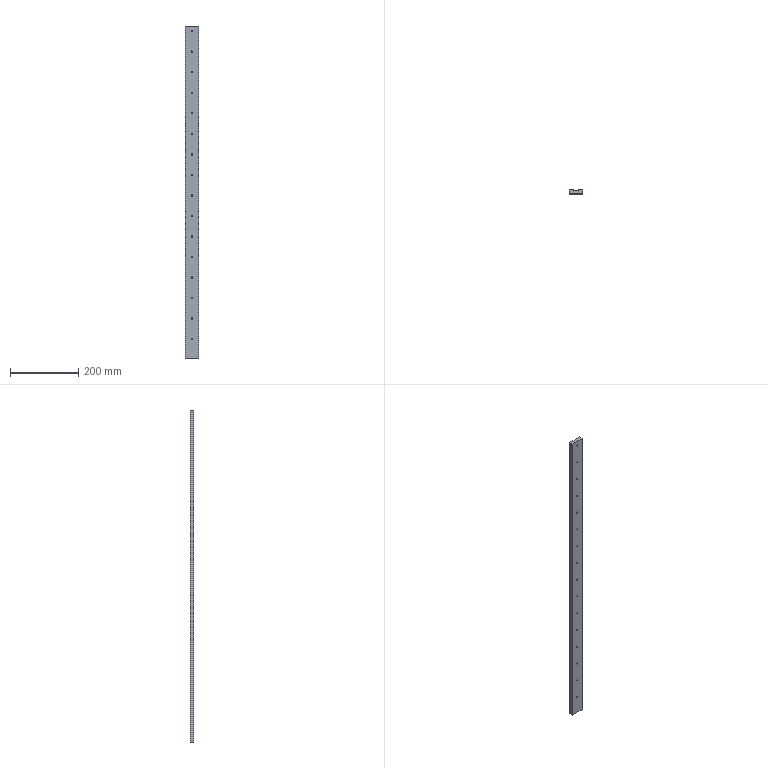Part | STEP file | X77-04205 | 1 solid | 42 faces | box 40 x 11 x 970 mm | volume 388716 mm3 | cylinder 32 | plane 10 | commonest cylinder face diameters 4 x32
STEP:
#1=CARTESIAN_POINT('',(-2.973,12.577,53.));
#2=VERTEX_POINT('',#1);
#3=CARTESIAN_POINT('',(-2.973,12.577,57.));
#4=VERTEX_POINT('',#3);
#5=CARTESIAN_POINT('',(-2.973,12.577,55.));
#6=DIRECTION('',(0.,1.,0.));
#7=DIRECTION('',(0.,0.,1.));
#8=AXIS2_PLACEMENT_3D('',#5,#6,#7);
#9=CIRCLE('',#8,2.);
#10=EDGE_CURVE('',#2,#4,#9,.T.);
#11=ORIENTED_EDGE('',*,*,#10,.F.);
#12=CARTESIAN_POINT('',(-2.973,21.077,53.));
#13=VERTEX_POINT('',#12);
#14=CARTESIAN_POINT('',(-2.973,21.077,53.));
#15=DIRECTION('',(0.,1.,0.));
#16=VECTOR('',#15,1000.);
#17=LINE('',#14,#16);
#18=EDGE_CURVE('',#2,#13,#17,.T.);
#19=ORIENTED_EDGE('',*,*,#18,.T.);
#20=CARTESIAN_POINT('',(-2.973,21.077,57.));
#21=VERTEX_POINT('',#20);
#22=CARTESIAN_POINT('',(-2.973,21.077,55.));
#23=DIRECTION('',(0.,1.,0.));
#24=DIRECTION('',(0.,0.,1.));
#25=AXIS2_PLACEMENT_3D('',#22,#23,#24);
#26=CIRCLE('',#25,2.);
#27=EDGE_CURVE('',#13,#21,#26,.T.);
#28=ORIENTED_EDGE('',*,*,#27,.T.);
#29=CARTESIAN_POINT('',(-2.973,21.077,57.));
#30=DIRECTION('',(0.,1.,0.));
#31=VECTOR('',#30,1000.);
#32=LINE('',#29,#31);
#33=EDGE_CURVE('',#4,#21,#32,.T.);
#34=ORIENTED_EDGE('',*,*,#33,.F.);
#35=EDGE_LOOP('',(#11,#19,#28,#34));
#36=FACE_OUTER_BOUND('',#35,.T.);
#37=CARTESIAN_POINT('',(-2.973,21.077,55.));
#38=DIRECTION('',(0.,1.,0.));
#39=DIRECTION('',(0.,0.,1.));
#40=AXIS2_PLACEMENT_3D('',#37,#38,#39);
#41=CYLINDRICAL_SURFACE('',#40,2.);
#42=ADVANCED_FACE('',(#36),#41,.F.);
#43=CARTESIAN_POINT('',(-2.973,12.577,113.));
#44=VERTEX_POINT('',#43);
#45=CARTESIAN_POINT('',(-2.973,12.577,117.));
#46=VERTEX_POINT('',#45);
#47=CARTESIAN_POINT('',(-2.973,12.577,115.));
#48=DIRECTION('',(0.,1.,0.));
#49=DIRECTION('',(0.,0.,1.));
#50=AXIS2_PLACEMENT_3D('',#47,#48,#49);
#51=CIRCLE('',#50,2.);
#52=EDGE_CURVE('',#44,#46,#51,.T.);
#53=ORIENTED_EDGE('',*,*,#52,.F.);
#54=CARTESIAN_POINT('',(-2.973,21.077,113.));
#55=VERTEX_POINT('',#54);
#56=CARTESIAN_POINT('',(-2.973,21.077,113.));
#57=DIRECTION('',(0.,1.,0.));
#58=VECTOR('',#57,1000.);
#59=LINE('',#56,#58);
#60=EDGE_CURVE('',#44,#55,#59,.T.);
#61=ORIENTED_EDGE('',*,*,#60,.T.);
#62=CARTESIAN_POINT('',(-2.973,21.077,117.));
#63=VERTEX_POINT('',#62);
#64=CARTESIAN_POINT('',(-2.973,21.077,115.));
#65=DIRECTION('',(0.,1.,0.));
#66=DIRECTION('',(0.,0.,1.));
#67=AXIS2_PLACEMENT_3D('',#64,#65,#66);
#68=CIRCLE('',#67,2.);
#69=EDGE_CURVE('',#55,#63,#68,.T.);
#70=ORIENTED_EDGE('',*,*,#69,.T.);
#71=CARTESIAN_POINT('',(-2.973,21.077,117.));
#72=DIRECTION('',(0.,1.,0.));
#73=VECTOR('',#72,1000.);
#74=LINE('',#71,#73);
#75=EDGE_CURVE('',#46,#63,#74,.T.);
#76=ORIENTED_EDGE('',*,*,#75,.F.);
#77=EDGE_LOOP('',(#53,#61,#70,#76));
#78=FACE_OUTER_BOUND('',#77,.T.);
#79=CARTESIAN_POINT('',(-2.973,21.077,115.));
#80=DIRECTION('',(0.,1.,0.));
#81=DIRECTION('',(0.,0.,1.));
#82=AXIS2_PLACEMENT_3D('',#79,#80,#81);
#83=CYLINDRICAL_SURFACE('',#82,2.);
#84=ADVANCED_FACE('',(#78),#83,.F.);
#85=CARTESIAN_POINT('',(-2.973,12.577,173.));
#86=VERTEX_POINT('',#85);
#87=CARTESIAN_POINT('',(-2.973,12.577,177.));
#88=VERTEX_POINT('',#87);
#89=CARTESIAN_POINT('',(-2.973,12.577,175.));
#90=DIRECTION('',(0.,1.,0.));
#91=DIRECTION('',(0.,0.,1.));
#92=AXIS2_PLACEMENT_3D('',#89,#90,#91);
#93=CIRCLE('',#92,2.);
#94=EDGE_CURVE('',#86,#88,#93,.T.);
#95=ORIENTED_EDGE('',*,*,#94,.F.);
#96=CARTESIAN_POINT('',(-2.973,21.077,173.));
#97=VERTEX_POINT('',#96);
#98=CARTESIAN_POINT('',(-2.973,21.077,173.));
#99=DIRECTION('',(0.,1.,0.));
#100=VECTOR('',#99,1000.);
#101=LINE('',#98,#100);
#102=EDGE_CURVE('',#86,#97,#101,.T.);
#103=ORIENTED_EDGE('',*,*,#102,.T.);
#104=CARTESIAN_POINT('',(-2.973,21.077,177.));
#105=VERTEX_POINT('',#104);
#106=CARTESIAN_POINT('',(-2.973,21.077,175.));
#107=DIRECTION('',(0.,1.,0.));
#108=DIRECTION('',(0.,0.,1.));
#109=AXIS2_PLACEMENT_3D('',#106,#107,#108);
#110=CIRCLE('',#109,2.);
#111=EDGE_CURVE('',#97,#105,#110,.T.);
#112=ORIENTED_EDGE('',*,*,#111,.T.);
#113=CARTESIAN_POINT('',(-2.973,21.077,177.));
#114=DIRECTION('',(0.,1.,0.));
#115=VECTOR('',#114,1000.);
#116=LINE('',#113,#115);
#117=EDGE_CURVE('',#88,#105,#116,.T.);
#118=ORIENTED_EDGE('',*,*,#117,.F.);
#119=EDGE_LOOP('',(#95,#103,#112,#118));
#120=FACE_OUTER_BOUND('',#119,.T.);
#121=CARTESIAN_POINT('',(-2.973,21.077,175.));
#122=DIRECTION('',(0.,1.,0.));
#123=DIRECTION('',(0.,0.,1.));
#124=AXIS2_PLACEMENT_3D('',#121,#122,#123);
#125=CYLINDRICAL_SURFACE('',#124,2.);
#126=ADVANCED_FACE('',(#120),#125,.F.);
#127=CARTESIAN_POINT('',(-2.973,12.577,233.));
#128=VERTEX_POINT('',#127);
#129=CARTESIAN_POINT('',(-2.973,12.577,237.));
#130=VERTEX_POINT('',#129);
#131=CARTESIAN_POINT('',(-2.973,12.577,235.));
#132=DIRECTION('',(0.,1.,0.));
#133=DIRECTION('',(0.,0.,1.));
#134=AXIS2_PLACEMENT_3D('',#131,#132,#133);
#135=CIRCLE('',#134,2.);
#136=EDGE_CURVE('',#128,#130,#135,.T.);
#137=ORIENTED_EDGE('',*,*,#136,.F.);
#138=CARTESIAN_POINT('',(-2.973,21.077,233.));
#139=VERTEX_POINT('',#138);
#140=CARTESIAN_POINT('',(-2.973,21.077,233.));
#141=DIRECTION('',(0.,1.,0.));
#142=VECTOR('',#141,1000.);
#143=LINE('',#140,#142);
#144=EDGE_CURVE('',#128,#139,#143,.T.);
#145=ORIENTED_EDGE('',*,*,#144,.T.);
#146=CARTESIAN_POINT('',(-2.973,21.077,237.));
#147=VERTEX_POINT('',#146);
#148=CARTESIAN_POINT('',(-2.973,21.077,235.));
#149=DIRECTION('',(0.,1.,0.));
#150=DIRECTION('',(0.,0.,1.));
#151=AXIS2_PLACEMENT_3D('',#148,#149,#150);
#152=CIRCLE('',#151,2.);
#153=EDGE_CURVE('',#139,#147,#152,.T.);
#154=ORIENTED_EDGE('',*,*,#153,.T.);
#155=CARTESIAN_POINT('',(-2.973,21.077,237.));
#156=DIRECTION('',(0.,1.,0.));
#157=VECTOR('',#156,1000.);
#158=LINE('',#155,#157);
#159=EDGE_CURVE('',#130,#147,#158,.T.);
#160=ORIENTED_EDGE('',*,*,#159,.F.);
#161=EDGE_LOOP('',(#137,#145,#154,#160));
#162=FACE_OUTER_BOUND('',#161,.T.);
#163=CARTESIAN_POINT('',(-2.973,21.077,235.));
#164=DIRECTION('',(0.,1.,0.));
#165=DIRECTION('',(0.,0.,1.));
#166=AXIS2_PLACEMENT_3D('',#163,#164,#165);
#167=CYLINDRICAL_SURFACE('',#166,2.);
#168=ADVANCED_FACE('',(#162),#167,.F.);
#169=CARTESIAN_POINT('',(-2.973,12.577,293.));
#170=VERTEX_POINT('',#169);
#171=CARTESIAN_POINT('',(-2.973,12.577,297.));
#172=VERTEX_POINT('',#171);
#173=CARTESIAN_POINT('',(-2.973,12.577,295.));
#174=DIRECTION('',(0.,1.,0.));
#175=DIRECTION('',(0.,0.,1.));
#176=AXIS2_PLACEMENT_3D('',#173,#174,#175);
#177=CIRCLE('',#176,2.);
#178=EDGE_CURVE('',#170,#172,#177,.T.);
#179=ORIENTED_EDGE('',*,*,#178,.F.);
#180=CARTESIAN_POINT('',(-2.973,21.077,293.));
#181=VERTEX_POINT('',#180);
#182=CARTESIAN_POINT('',(-2.973,21.077,293.));
#183=DIRECTION('',(0.,1.,0.));
#184=VECTOR('',#183,1000.);
#185=LINE('',#182,#184);
#186=EDGE_CURVE('',#170,#181,#185,.T.);
#187=ORIENTED_EDGE('',*,*,#186,.T.);
#188=CARTESIAN_POINT('',(-2.973,21.077,297.));
#189=VERTEX_POINT('',#188);
#190=CARTESIAN_POINT('',(-2.973,21.077,295.));
#191=DIRECTION('',(0.,1.,0.));
#192=DIRECTION('',(0.,0.,1.));
#193=AXIS2_PLACEMENT_3D('',#190,#191,#192);
#194=CIRCLE('',#193,2.);
#195=EDGE_CURVE('',#181,#189,#194,.T.);
#196=ORIENTED_EDGE('',*,*,#195,.T.);
#197=CARTESIAN_POINT('',(-2.973,21.077,297.));
#198=DIRECTION('',(0.,1.,0.));
#199=VECTOR('',#198,1000.);
#200=LINE('',#197,#199);
#201=EDGE_CURVE('',#172,#189,#200,.T.);
#202=ORIENTED_EDGE('',*,*,#201,.F.);
#203=EDGE_LOOP('',(#179,#187,#196,#202));
#204=FACE_OUTER_BOUND('',#203,.T.);
#205=CARTESIAN_POINT('',(-2.973,21.077,295.));
#206=DIRECTION('',(0.,1.,0.));
#207=DIRECTION('',(0.,0.,1.));
#208=AXIS2_PLACEMENT_3D('',#205,#206,#207);
#209=CYLINDRICAL_SURFACE('',#208,2.);
#210=ADVANCED_FACE('',(#204),#209,.F.);
#211=CARTESIAN_POINT('',(-2.973,12.577,353.));
#212=VERTEX_POINT('',#211);
#213=CARTESIAN_POINT('',(-2.973,12.577,357.));
#214=VERTEX_POINT('',#213);
#215=CARTESIAN_POINT('',(-2.973,12.577,355.));
#216=DIRECTION('',(0.,1.,0.));
#217=DIRECTION('',(0.,0.,1.));
#218=AXIS2_PLACEMENT_3D('',#215,#216,#217);
#219=CIRCLE('',#218,2.);
#220=EDGE_CURVE('',#212,#214,#219,.T.);
#221=ORIENTED_EDGE('',*,*,#220,.F.);
#222=CARTESIAN_POINT('',(-2.973,21.077,353.));
#223=VERTEX_POINT('',#222);
#224=CARTESIAN_POINT('',(-2.973,21.077,353.));
#225=DIRECTION('',(0.,1.,0.));
#226=VECTOR('',#225,1000.);
#227=LINE('',#224,#226);
#228=EDGE_CURVE('',#212,#223,#227,.T.);
#229=ORIENTED_EDGE('',*,*,#228,.T.);
#230=CARTESIAN_POINT('',(-2.973,21.077,357.));
#231=VERTEX_POINT('',#230);
#232=CARTESIAN_POINT('',(-2.973,21.077,355.));
#233=DIRECTION('',(0.,1.,0.));
#234=DIRECTION('',(0.,0.,1.));
#235=AXIS2_PLACEMENT_3D('',#232,#233,#234);
#236=CIRCLE('',#235,2.);
#237=EDGE_CURVE('',#223,#231,#236,.T.);
#238=ORIENTED_EDGE('',*,*,#237,.T.);
#239=CARTESIAN_POINT('',(-2.973,21.077,357.));
#240=DIRECTION('',(0.,1.,0.));
#241=VECTOR('',#240,1000.);
#242=LINE('',#239,#241);
#243=EDGE_CURVE('',#214,#231,#242,.T.);
#244=ORIENTED_EDGE('',*,*,#243,.F.);
#245=EDGE_LOOP('',(#221,#229,#238,#244));
#246=FACE_OUTER_BOUND('',#245,.T.);
#247=CARTESIAN_POINT('',(-2.973,21.077,355.));
#248=DIRECTION('',(0.,1.,0.));
#249=DIRECTION('',(0.,0.,1.));
#250=AXIS2_PLACEMENT_3D('',#247,#248,#249);
#251=CYLINDRICAL_SURFACE('',#250,2.);
#252=ADVANCED_FACE('',(#246),#251,.F.);
#253=CARTESIAN_POINT('',(-2.973,12.577,413.));
#254=VERTEX_POINT('',#253);
#255=CARTESIAN_POINT('',(-2.973,12.577,417.));
#256=VERTEX_POINT('',#255);
#257=CARTESIAN_POINT('',(-2.973,12.577,415.));
#258=DIRECTION('',(0.,1.,0.));
#259=DIRECTION('',(0.,0.,1.));
#260=AXIS2_PLACEMENT_3D('',#257,#258,#259);
#261=CIRCLE('',#260,2.);
#262=EDGE_CURVE('',#254,#256,#261,.T.);
#263=ORIENTED_EDGE('',*,*,#262,.F.);
#264=CARTESIAN_POINT('',(-2.973,21.077,413.));
#265=VERTEX_POINT('',#264);
#266=CARTESIAN_POINT('',(-2.973,21.077,413.));
#267=DIRECTION('',(0.,1.,0.));
#268=VECTOR('',#267,1000.);
#269=LINE('',#266,#268);
#270=EDGE_CURVE('',#254,#265,#269,.T.);
#271=ORIENTED_EDGE('',*,*,#270,.T.);
#272=CARTESIAN_POINT('',(-2.973,21.077,417.));
#273=VERTEX_POINT('',#272);
#274=CARTESIAN_POINT('',(-2.973,21.077,415.));
#275=DIRECTION('',(0.,1.,0.));
#276=DIRECTION('',(0.,0.,1.));
#277=AXIS2_PLACEMENT_3D('',#274,#275,#276);
#278=CIRCLE('',#277,2.);
#279=EDGE_CURVE('',#265,#273,#278,.T.);
#280=ORIENTED_EDGE('',*,*,#279,.T.);
#281=CARTESIAN_POINT('',(-2.973,21.077,417.));
#282=DIRECTION('',(0.,1.,0.));
#283=VECTOR('',#282,1000.);
#284=LINE('',#281,#283);
#285=EDGE_CURVE('',#256,#273,#284,.T.);
#286=ORIENTED_EDGE('',*,*,#285,.F.);
#287=EDGE_LOOP('',(#263,#271,#280,#286));
#288=FACE_OUTER_BOUND('',#287,.T.);
#289=CARTESIAN_POINT('',(-2.973,21.077,415.));
#290=DIRECTION('',(0.,1.,0.));
#291=DIRECTION('',(0.,0.,1.));
#292=AXIS2_PLACEMENT_3D('',#289,#290,#291);
#293=CYLINDRICAL_SURFACE('',#292,2.);
#294=ADVANCED_FACE('',(#288),#293,.F.);
#295=CARTESIAN_POINT('',(-2.973,12.577,473.));
#296=VERTEX_POINT('',#295);
#297=CARTESIAN_POINT('',(-2.973,12.577,477.));
#298=VERTEX_POINT('',#297);
#299=CARTESIAN_POINT('',(-2.973,12.577,475.));
#300=DIRECTION('',(0.,1.,0.));
#301=DIRECTION('',(0.,0.,1.));
#302=AXIS2_PLACEMENT_3D('',#299,#300,#301);
#303=CIRCLE('',#302,2.);
#304=EDGE_CURVE('',#296,#298,#303,.T.);
#305=ORIENTED_EDGE('',*,*,#304,.F.);
#306=CARTESIAN_POINT('',(-2.973,21.077,473.));
#307=VERTEX_POINT('',#306);
#308=CARTESIAN_POINT('',(-2.973,21.077,473.));
#309=DIRECTION('',(0.,1.,0.));
#310=VECTOR('',#309,1000.);
#311=LINE('',#308,#310);
#312=EDGE_CURVE('',#296,#307,#311,.T.);
#313=ORIENTED_EDGE('',*,*,#312,.T.);
#314=CARTESIAN_POINT('',(-2.973,21.077,477.));
#315=VERTEX_POINT('',#314);
#316=CARTESIAN_POINT('',(-2.973,21.077,475.));
#317=DIRECTION('',(0.,1.,0.));
#318=DIRECTION('',(0.,0.,1.));
#319=AXIS2_PLACEMENT_3D('',#316,#317,#318);
#320=CIRCLE('',#319,2.);
#321=EDGE_CURVE('',#307,#315,#320,.T.);
#322=ORIENTED_EDGE('',*,*,#321,.T.);
#323=CARTESIAN_POINT('',(-2.973,21.077,477.));
#324=DIRECTION('',(0.,1.,0.));
#325=VECTOR('',#324,1000.);
#326=LINE('',#323,#325);
#327=EDGE_CURVE('',#298,#315,#326,.T.);
#328=ORIENTED_EDGE('',*,*,#327,.F.);
#329=EDGE_LOOP('',(#305,#313,#322,#328));
#330=FACE_OUTER_BOUND('',#329,.T.);
#331=CARTESIAN_POINT('',(-2.973,21.077,475.));
#332=DIRECTION('',(0.,1.,0.));
#333=DIRECTION('',(0.,0.,1.));
#334=AXIS2_PLACEMENT_3D('',#331,#332,#333);
#335=CYLINDRICAL_SURFACE('',#334,2.);
#336=ADVANCED_FACE('',(#330),#335,.F.);
#337=CARTESIAN_POINT('',(-2.973,12.577,533.));
#338=VERTEX_POINT('',#337);
#339=CARTESIAN_POINT('',(-2.973,12.577,537.));
#340=VERTEX_POINT('',#339);
#341=CARTESIAN_POINT('',(-2.973,12.577,535.));
#342=DIRECTION('',(0.,1.,0.));
#343=DIRECTION('',(0.,0.,1.));
#344=AXIS2_PLACEMENT_3D('',#341,#342,#343);
#345=CIRCLE('',#344,2.);
#346=EDGE_CURVE('',#338,#340,#345,.T.);
#347=ORIENTED_EDGE('',*,*,#346,.F.);
#348=CARTESIAN_POINT('',(-2.973,21.077,533.));
#349=VERTEX_POINT('',#348);
#350=CARTESIAN_POINT('',(-2.973,21.077,533.));
#351=DIRECTION('',(0.,1.,0.));
#352=VECTOR('',#351,1000.);
#353=LINE('',#350,#352);
#354=EDGE_CURVE('',#338,#349,#353,.T.);
#355=ORIENTED_EDGE('',*,*,#354,.T.);
#356=CARTESIAN_POINT('',(-2.973,21.077,537.));
#357=VERTEX_POINT('',#356);
#358=CARTESIAN_POINT('',(-2.973,21.077,535.));
#359=DIRECTION('',(0.,1.,0.));
#360=DIRECTION('',(0.,0.,1.));
#361=AXIS2_PLACEMENT_3D('',#358,#359,#360);
#362=CIRCLE('',#361,2.);
#363=EDGE_CURVE('',#349,#357,#362,.T.);
#364=ORIENTED_EDGE('',*,*,#363,.T.);
#365=CARTESIAN_POINT('',(-2.973,21.077,537.));
#366=DIRECTION('',(0.,1.,0.));
#367=VECTOR('',#366,1000.);
#368=LINE('',#365,#367);
#369=EDGE_CURVE('',#340,#357,#368,.T.);
#370=ORIENTED_EDGE('',*,*,#369,.F.);
#371=EDGE_LOOP('',(#347,#355,#364,#370));
#372=FACE_OUTER_BOUND('',#371,.T.);
#373=CARTESIAN_POINT('',(-2.973,21.077,535.));
#374=DIRECTION('',(0.,1.,0.));
#375=DIRECTION('',(0.,0.,1.));
#376=AXIS2_PLACEMENT_3D('',#373,#374,#375);
#377=CYLINDRICAL_SURFACE('',#376,2.);
#378=ADVANCED_FACE('',(#372),#377,.F.);
#379=CARTESIAN_POINT('',(-2.973,12.577,593.));
#380=VERTEX_POINT('',#379);
#381=CARTESIAN_POINT('',(-2.973,12.577,597.));
#382=VERTEX_POINT('',#381);
#383=CARTESIAN_POINT('',(-2.973,12.577,595.));
#384=DIRECTION('',(0.,1.,0.));
#385=DIRECTION('',(0.,0.,1.));
#386=AXIS2_PLACEMENT_3D('',#383,#384,#385);
#387=CIRCLE('',#386,2.);
#388=EDGE_CURVE('',#380,#382,#387,.T.);
#389=ORIENTED_EDGE('',*,*,#388,.F.);
#390=CARTESIAN_POINT('',(-2.973,21.077,593.));
#391=VERTEX_POINT('',#390);
#392=CARTESIAN_POINT('',(-2.973,21.077,593.));
#393=DIRECTION('',(0.,1.,0.));
#394=VECTOR('',#393,1000.);
#395=LINE('',#392,#394);
#396=EDGE_CURVE('',#380,#391,#395,.T.);
#397=ORIENTED_EDGE('',*,*,#396,.T.);
#398=CARTESIAN_POINT('',(-2.973,21.077,597.));
#399=VERTEX_POINT('',#398);
#400=CARTESIAN_POINT('',(-2.973,21.077,595.));
#401=DIRECTION('',(0.,1.,0.));
#402=DIRECTION('',(0.,0.,1.));
#403=AXIS2_PLACEMENT_3D('',#400,#401,#402);
#404=CIRCLE('',#403,2.);
#405=EDGE_CURVE('',#391,#399,#404,.T.);
#406=ORIENTED_EDGE('',*,*,#405,.T.);
#407=CARTESIAN_POINT('',(-2.973,21.077,597.));
#408=DIRECTION('',(0.,1.,0.));
#409=VECTOR('',#408,1000.);
#410=LINE('',#407,#409);
#411=EDGE_CURVE('',#382,#399,#410,.T.);
#412=ORIENTED_EDGE('',*,*,#411,.F.);
#413=EDGE_LOOP('',(#389,#397,#406,#412));
#414=FACE_OUTER_BOUND('',#413,.T.);
#415=CARTESIAN_POINT('',(-2.973,21.077,595.));
#416=DIRECTION('',(0.,1.,0.));
#417=DIRECTION('',(0.,0.,1.));
#418=AXIS2_PLACEMENT_3D('',#415,#416,#417);
#419=CYLINDRICAL_SURFACE('',#418,2.);
#420=ADVANCED_FACE('',(#414),#419,.F.);
#421=CARTESIAN_POINT('',(-2.973,12.577,653.));
#422=VERTEX_POINT('',#421);
#423=CARTESIAN_POINT('',(-2.973,12.577,657.));
#424=VERTEX_POINT('',#423);
#425=CARTESIAN_POINT('',(-2.973,12.577,655.));
#426=DIRECTION('',(0.,1.,0.));
#427=DIRECTION('',(0.,0.,1.));
#428=AXIS2_PLACEMENT_3D('',#425,#426,#427);
#429=CIRCLE('',#428,2.);
#430=EDGE_CURVE('',#422,#424,#429,.T.);
#431=ORIENTED_EDGE('',*,*,#430,.F.);
#432=CARTESIAN_POINT('',(-2.973,21.077,653.));
#433=VERTEX_POINT('',#432);
#434=CARTESIAN_POINT('',(-2.973,21.077,653.));
#435=DIRECTION('',(0.,1.,0.));
#436=VECTOR('',#435,1000.);
#437=LINE('',#434,#436);
#438=EDGE_CURVE('',#422,#433,#437,.T.);
#439=ORIENTED_EDGE('',*,*,#438,.T.);
#440=CARTESIAN_POINT('',(-2.973,21.077,657.));
#441=VERTEX_POINT('',#440);
#442=CARTESIAN_POINT('',(-2.973,21.077,655.));
#443=DIRECTION('',(0.,1.,0.));
#444=DIRECTION('',(0.,0.,1.));
#445=AXIS2_PLACEMENT_3D('',#442,#443,#444);
#446=CIRCLE('',#445,2.);
#447=EDGE_CURVE('',#433,#441,#446,.T.);
#448=ORIENTED_EDGE('',*,*,#447,.T.);
#449=CARTESIAN_POINT('',(-2.973,21.077,657.));
#450=DIRECTION('',(0.,1.,0.));
#451=VECTOR('',#450,1000.);
#452=LINE('',#449,#451);
#453=EDGE_CURVE('',#424,#441,#452,.T.);
#454=ORIENTED_EDGE('',*,*,#453,.F.);
#455=EDGE_LOOP('',(#431,#439,#448,#454));
#456=FACE_OUTER_BOUND('',#455,.T.);
#457=CARTESIAN_POINT('',(-2.973,21.077,655.));
#458=DIRECTION('',(0.,1.,0.));
#459=DIRECTION('',(0.,0.,1.));
#460=AXIS2_PLACEMENT_3D('',#457,#458,#459);
#461=CYLINDRICAL_SURFACE('',#460,2.);
#462=ADVANCED_FACE('',(#456),#461,.F.);
#463=CARTESIAN_POINT('',(-2.973,12.577,713.));
#464=VERTEX_POINT('',#463);
#465=CARTESIAN_POINT('',(-2.973,12.577,717.));
#466=VERTEX_POINT('',#465);
#467=CARTESIAN_POINT('',(-2.973,12.577,715.));
#468=DIRECTION('',(0.,1.,0.));
#469=DIRECTION('',(0.,0.,1.));
#470=AXIS2_PLACEMENT_3D('',#467,#468,#469);
#471=CIRCLE('',#470,2.);
#472=EDGE_CURVE('',#464,#466,#471,.T.);
#473=ORIENTED_EDGE('',*,*,#472,.F.);
#474=CARTESIAN_POINT('',(-2.973,21.077,713.));
#475=VERTEX_POINT('',#474);
#476=CARTESIAN_POINT('',(-2.973,21.077,713.));
#477=DIRECTION('',(0.,1.,0.));
#478=VECTOR('',#477,1000.);
#479=LINE('',#476,#478);
#480=EDGE_CURVE('',#464,#475,#479,.T.);
#481=ORIENTED_EDGE('',*,*,#480,.T.);
#482=CARTESIAN_POINT('',(-2.973,21.077,717.));
#483=VERTEX_POINT('',#482);
#484=CARTESIAN_POINT('',(-2.973,21.077,715.));
#485=DIRECTION('',(0.,1.,0.));
#486=DIRECTION('',(0.,0.,1.));
#487=AXIS2_PLACEMENT_3D('',#484,#485,#486);
#488=CIRCLE('',#487,2.);
#489=EDGE_CURVE('',#475,#483,#488,.T.);
#490=ORIENTED_EDGE('',*,*,#489,.T.);
#491=CARTESIAN_POINT('',(-2.973,21.077,717.));
#492=DIRECTION('',(0.,1.,0.));
#493=VECTOR('',#492,1000.);
#494=LINE('',#491,#493);
#495=EDGE_CURVE('',#466,#483,#494,.T.);
#496=ORIENTED_EDGE('',*,*,#495,.F.);
#497=EDGE_LOOP('',(#473,#481,#490,#496));
#498=FACE_OUTER_BOUND('',#497,.T.);
#499=CARTESIAN_POINT('',(-2.973,21.077,715.));
#500=DIRECTION('',(0.,1.,0.));
#501=DIRECTION('',(0.,0.,1.));
#502=AXIS2_PLACEMENT_3D('',#499,#500,#501);
#503=CYLINDRICAL_SURFACE('',#502,2.);
#504=ADVANCED_FACE('',(#498),#503,.F.);
#505=CARTESIAN_POINT('',(-2.973,12.577,773.));
#506=VERTEX_POINT('',#505);
#507=CARTESIAN_POINT('',(-2.973,12.577,777.));
#508=VERTEX_POINT('',#507);
#509=CARTESIAN_POINT('',(-2.973,12.577,775.));
#510=DIRECTION('',(0.,1.,0.));
#511=DIRECTION('',(0.,0.,1.));
#512=AXIS2_PLACEMENT_3D('',#509,#510,#511);
#513=CIRCLE('',#512,2.);
#514=EDGE_CURVE('',#506,#508,#513,.T.);
#515=ORIENTED_EDGE('',*,*,#514,.F.);
#516=CARTESIAN_POINT('',(-2.973,21.077,773.));
#517=VERTEX_POINT('',#516);
#518=CARTESIAN_POINT('',(-2.973,21.077,773.));
#519=DIRECTION('',(0.,1.,0.));
#520=VECTOR('',#519,1000.);
#521=LINE('',#518,#520);
#522=EDGE_CURVE('',#506,#517,#521,.T.);
#523=ORIENTED_EDGE('',*,*,#522,.T.);
#524=CARTESIAN_POINT('',(-2.973,21.077,777.));
#525=VERTEX_POINT('',#524);
#526=CARTESIAN_POINT('',(-2.973,21.077,775.));
#527=DIRECTION('',(0.,1.,0.));
#528=DIRECTION('',(0.,0.,1.));
#529=AXIS2_PLACEMENT_3D('',#526,#527,#528);
#530=CIRCLE('',#529,2.);
#531=EDGE_CURVE('',#517,#525,#530,.T.);
#532=ORIENTED_EDGE('',*,*,#531,.T.);
#533=CARTESIAN_POINT('',(-2.973,21.077,777.));
#534=DIRECTION('',(0.,1.,0.));
#535=VECTOR('',#534,1000.);
#536=LINE('',#533,#535);
#537=EDGE_CURVE('',#508,#525,#536,.T.);
#538=ORIENTED_EDGE('',*,*,#537,.F.);
#539=EDGE_LOOP('',(#515,#523,#532,#538));
#540=FACE_OUTER_BOUND('',#539,.T.);
#541=CARTESIAN_POINT('',(-2.973,21.077,775.));
#542=DIRECTION('',(0.,1.,0.));
#543=DIRECTION('',(0.,0.,1.));
#544=AXIS2_PLACEMENT_3D('',#541,#542,#543);
#545=CYLINDRICAL_SURFACE('',#544,2.);
#546=ADVANCED_FACE('',(#540),#545,.F.);
#547=CARTESIAN_POINT('',(-2.973,12.577,833.));
#548=VERTEX_POINT('',#547);
#549=CARTESIAN_POINT('',(-2.973,12.577,837.));
#550=VERTEX_POINT('',#549);
#551=CARTESIAN_POINT('',(-2.973,12.577,835.));
#552=DIRECTION('',(0.,1.,0.));
#553=DIRECTION('',(0.,0.,1.));
#554=AXIS2_PLACEMENT_3D('',#551,#552,#553);
#555=CIRCLE('',#554,2.);
#556=EDGE_CURVE('',#548,#550,#555,.T.);
#557=ORIENTED_EDGE('',*,*,#556,.F.);
#558=CARTESIAN_POINT('',(-2.973,21.077,833.));
#559=VERTEX_POINT('',#558);
#560=CARTESIAN_POINT('',(-2.973,21.077,833.));
#561=DIRECTION('',(0.,1.,0.));
#562=VECTOR('',#561,1000.);
#563=LINE('',#560,#562);
#564=EDGE_CURVE('',#548,#559,#563,.T.);
#565=ORIENTED_EDGE('',*,*,#564,.T.);
#566=CARTESIAN_POINT('',(-2.973,21.077,837.));
#567=VERTEX_POINT('',#566);
#568=CARTESIAN_POINT('',(-2.973,21.077,835.));
#569=DIRECTION('',(0.,1.,0.));
#570=DIRECTION('',(0.,0.,1.));
#571=AXIS2_PLACEMENT_3D('',#568,#569,#570);
#572=CIRCLE('',#571,2.);
#573=EDGE_CURVE('',#559,#567,#572,.T.);
#574=ORIENTED_EDGE('',*,*,#573,.T.);
#575=CARTESIAN_POINT('',(-2.973,21.077,837.));
#576=DIRECTION('',(0.,1.,0.));
#577=VECTOR('',#576,1000.);
#578=LINE('',#575,#577);
#579=EDGE_CURVE('',#550,#567,#578,.T.);
#580=ORIENTED_EDGE('',*,*,#579,.F.);
#581=EDGE_LOOP('',(#557,#565,#574,#580));
#582=FACE_OUTER_BOUND('',#581,.T.);
#583=CARTESIAN_POINT('',(-2.973,21.077,835.));
#584=DIRECTION('',(0.,1.,0.));
#585=DIRECTION('',(0.,0.,1.));
#586=AXIS2_PLACEMENT_3D('',#583,#584,#585);
#587=CYLINDRICAL_SURFACE('',#586,2.);
#588=ADVANCED_FACE('',(#582),#587,.F.);
#589=CARTESIAN_POINT('',(-2.973,12.577,893.));
#590=VERTEX_POINT('',#589);
#591=CARTESIAN_POINT('',(-2.973,12.577,897.));
#592=VERTEX_POINT('',#591);
#593=CARTESIAN_POINT('',(-2.973,12.577,895.));
#594=DIRECTION('',(0.,1.,0.));
#595=DIRECTION('',(0.,0.,1.));
#596=AXIS2_PLACEMENT_3D('',#593,#594,#595);
#597=CIRCLE('',#596,2.);
#598=EDGE_CURVE('',#590,#592,#597,.T.);
#599=ORIENTED_EDGE('',*,*,#598,.F.);
#600=CARTESIAN_POINT('',(-2.973,21.077,893.));
#601=VERTEX_POINT('',#600);
#602=CARTESIAN_POINT('',(-2.973,21.077,893.));
#603=DIRECTION('',(0.,1.,0.));
#604=VECTOR('',#603,1000.);
#605=LINE('',#602,#604);
#606=EDGE_CURVE('',#590,#601,#605,.T.);
#607=ORIENTED_EDGE('',*,*,#606,.T.);
#608=CARTESIAN_POINT('',(-2.973,21.077,897.));
#609=VERTEX_POINT('',#608);
#610=CARTESIAN_POINT('',(-2.973,21.077,895.));
#611=DIRECTION('',(0.,1.,0.));
#612=DIRECTION('',(0.,0.,1.));
#613=AXIS2_PLACEMENT_3D('',#610,#611,#612);
#614=CIRCLE('',#613,2.);
#615=EDGE_CURVE('',#601,#609,#614,.T.);
#616=ORIENTED_EDGE('',*,*,#615,.T.);
#617=CARTESIAN_POINT('',(-2.973,21.077,897.));
#618=DIRECTION('',(0.,1.,0.));
#619=VECTOR('',#618,1000.);
#620=LINE('',#617,#619);
#621=EDGE_CURVE('',#592,#609,#620,.T.);
#622=ORIENTED_EDGE('',*,*,#621,.F.);
#623=EDGE_LOOP('',(#599,#607,#616,#622));
#624=FACE_OUTER_BOUND('',#623,.T.);
#625=CARTESIAN_POINT('',(-2.973,21.077,895.));
#626=DIRECTION('',(0.,1.,0.));
#627=DIRECTION('',(0.,0.,1.));
#628=AXIS2_PLACEMENT_3D('',#625,#626,#627);
#629=CYLINDRICAL_SURFACE('',#628,2.);
#630=ADVANCED_FACE('',(#624),#629,.F.);
#631=CARTESIAN_POINT('',(-2.973,12.577,953.));
#632=VERTEX_POINT('',#631);
#633=CARTESIAN_POINT('',(-2.973,12.577,957.));
#634=VERTEX_POINT('',#633);
#635=CARTESIAN_POINT('',(-2.973,12.577,955.));
#636=DIRECTION('',(0.,1.,0.));
#637=DIRECTION('',(0.,0.,1.));
#638=AXIS2_PLACEMENT_3D('',#635,#636,#637);
#639=CIRCLE('',#638,2.);
#640=EDGE_CURVE('',#632,#634,#639,.T.);
#641=ORIENTED_EDGE('',*,*,#640,.F.);
#642=CARTESIAN_POINT('',(-2.973,21.077,953.));
#643=VERTEX_POINT('',#642);
#644=CARTESIAN_POINT('',(-2.973,21.077,953.));
#645=DIRECTION('',(0.,1.,0.));
#646=VECTOR('',#645,1000.);
#647=LINE('',#644,#646);
#648=EDGE_CURVE('',#632,#643,#647,.T.);
#649=ORIENTED_EDGE('',*,*,#648,.T.);
#650=CARTESIAN_POINT('',(-2.973,21.077,957.));
#651=VERTEX_POINT('',#650);
#652=CARTESIAN_POINT('',(-2.973,21.077,955.));
#653=DIRECTION('',(0.,1.,0.));
#654=DIRECTION('',(0.,0.,1.));
#655=AXIS2_PLACEMENT_3D('',#652,#653,#654);
#656=CIRCLE('',#655,2.);
#657=EDGE_CURVE('',#643,#651,#656,.T.);
#658=ORIENTED_EDGE('',*,*,#657,.T.);
#659=CARTESIAN_POINT('',(-2.973,21.077,957.));
#660=DIRECTION('',(0.,1.,0.));
#661=VECTOR('',#660,1000.);
#662=LINE('',#659,#661);
#663=EDGE_CURVE('',#634,#651,#662,.T.);
#664=ORIENTED_EDGE('',*,*,#663,.F.);
#665=EDGE_LOOP('',(#641,#649,#658,#664));
#666=FACE_OUTER_BOUND('',#665,.T.);
#667=CARTESIAN_POINT('',(-2.973,21.077,955.));
#668=DIRECTION('',(0.,1.,0.));
#669=DIRECTION('',(0.,0.,1.));
#670=AXIS2_PLACEMENT_3D('',#667,#668,#669);
#671=CYLINDRICAL_SURFACE('',#670,2.);
#672=ADVANCED_FACE('',(#666),#671,.F.);
#673=CARTESIAN_POINT('',(17.027,23.577,0.));
#674=VERTEX_POINT('',#673);
#675=CARTESIAN_POINT('',(4.527,23.577,0.));
#676=VERTEX_POINT('',#675);
#677=CARTESIAN_POINT('',(-22.973,23.577,0.));
#678=DIRECTION('',(-1.,0.,0.));
#679=VECTOR('',#678,1000.);
#680=LINE('',#677,#679);
#681=EDGE_CURVE('',#674,#676,#680,.T.);
#682=ORIENTED_EDGE('',*,*,#681,.T.);
#683=CARTESIAN_POINT('',(4.527,23.577,970.));
#684=VERTEX_POINT('',#683);
#685=CARTESIAN_POINT('',(4.527,23.577,0.));
#686=DIRECTION('',(0.,0.,1.));
#687=VECTOR('',#686,1000.);
#688=LINE('',#685,#687);
#689=EDGE_CURVE('',#676,#684,#688,.T.);
#690=ORIENTED_EDGE('',*,*,#689,.T.);
#691=CARTESIAN_POINT('',(17.027,23.577,970.));
#692=VERTEX_POINT('',#691);
#693=CARTESIAN_POINT('',(-22.973,23.577,970.));
#694=DIRECTION('',(-1.,0.,0.));
#695=VECTOR('',#694,1000.);
#696=LINE('',#693,#695);
#697=EDGE_CURVE('',#692,#684,#696,.T.);
#698=ORIENTED_EDGE('',*,*,#697,.F.);
#699=CARTESIAN_POINT('',(17.027,23.577,970.));
#700=DIRECTION('',(0.,0.,-1.));
#701=VECTOR('',#700,1000.);
#702=LINE('',#699,#701);
#703=EDGE_CURVE('',#692,#674,#702,.T.);
#704=ORIENTED_EDGE('',*,*,#703,.T.);
#705=EDGE_LOOP('',(#682,#690,#698,#704));
#706=FACE_OUTER_BOUND('',#705,.T.);
#707=CARTESIAN_POINT('',(-22.973,23.577,970.));
#708=DIRECTION('',(0.,-1.,0.));
#709=DIRECTION('',(0.,0.,-1.));
#710=AXIS2_PLACEMENT_3D('',#707,#708,#709);
#711=PLANE('',#710);
#712=ADVANCED_FACE('',(#706),#711,.F.);
#713=CARTESIAN_POINT('',(-22.973,23.577,0.));
#714=VERTEX_POINT('',#713);
#715=CARTESIAN_POINT('',(-22.973,12.577,0.));
#716=VERTEX_POINT('',#715);
#717=CARTESIAN_POINT('',(-22.973,12.577,0.));
#718=DIRECTION('',(0.,-1.,0.));
#719=VECTOR('',#718,1000.);
#720=LINE('',#717,#719);
#721=EDGE_CURVE('',#714,#716,#720,.T.);
#722=ORIENTED_EDGE('',*,*,#721,.T.);
#723=CARTESIAN_POINT('',(-22.973,12.577,970.));
#724=VERTEX_POINT('',#723);
#725=CARTESIAN_POINT('',(-22.973,12.577,970.));
#726=DIRECTION('',(0.,0.,-1.));
#727=VECTOR('',#726,1000.);
#728=LINE('',#725,#727);
#729=EDGE_CURVE('',#724,#716,#728,.T.);
#730=ORIENTED_EDGE('',*,*,#729,.F.);
#731=CARTESIAN_POINT('',(-22.973,23.577,970.));
#732=VERTEX_POINT('',#731);
#733=CARTESIAN_POINT('',(-22.973,12.577,970.));
#734=DIRECTION('',(0.,-1.,0.));
#735=VECTOR('',#734,1000.);
#736=LINE('',#733,#735);
#737=EDGE_CURVE('',#732,#724,#736,.T.);
#738=ORIENTED_EDGE('',*,*,#737,.F.);
#739=CARTESIAN_POINT('',(-22.973,23.577,970.));
#740=DIRECTION('',(0.,0.,-1.));
#741=VECTOR('',#740,1000.);
#742=LINE('',#739,#741);
#743=EDGE_CURVE('',#732,#714,#742,.T.);
#744=ORIENTED_EDGE('',*,*,#743,.T.);
#745=EDGE_LOOP('',(#722,#730,#738,#744));
#746=FACE_OUTER_BOUND('',#745,.T.);
#747=CARTESIAN_POINT('',(-22.973,12.577,970.));
#748=DIRECTION('',(1.,0.,0.));
#749=DIRECTION('',(0.,0.,-1.));
#750=AXIS2_PLACEMENT_3D('',#747,#748,#749);
#751=PLANE('',#750);
#752=ADVANCED_FACE('',(#746),#751,.F.);
#753=CARTESIAN_POINT('',(-2.973,12.577,895.));
#754=DIRECTION('',(0.,1.,0.));
#755=DIRECTION('',(0.,0.,1.));
#756=AXIS2_PLACEMENT_3D('',#753,#754,#755);
#757=CIRCLE('',#756,2.);
#758=EDGE_CURVE('',#592,#590,#757,.T.);
#759=ORIENTED_EDGE('',*,*,#758,.T.);
#760=ORIENTED_EDGE('',*,*,#598,.T.);
#761=EDGE_LOOP('',(#759,#760));
#762=FACE_BOUND('',#761,.T.);
#763=CARTESIAN_POINT('',(-2.973,12.577,955.));
#764=DIRECTION('',(0.,1.,0.));
#765=DIRECTION('',(0.,0.,1.));
#766=AXIS2_PLACEMENT_3D('',#763,#764,#765);
#767=CIRCLE('',#766,2.);
#768=EDGE_CURVE('',#634,#632,#767,.T.);
#769=ORIENTED_EDGE('',*,*,#768,.T.);
#770=ORIENTED_EDGE('',*,*,#640,.T.);
#771=EDGE_LOOP('',(#769,#770));
#772=FACE_BOUND('',#771,.T.);
#773=CARTESIAN_POINT('',(17.027,12.577,0.));
#774=VERTEX_POINT('',#773);
#775=CARTESIAN_POINT('',(-22.973,12.577,0.));
#776=DIRECTION('',(1.,0.,0.));
#777=VECTOR('',#776,1000.);
#778=LINE('',#775,#777);
#779=EDGE_CURVE('',#716,#774,#778,.T.);
#780=ORIENTED_EDGE('',*,*,#779,.T.);
#781=CARTESIAN_POINT('',(17.027,12.577,970.));
#782=VERTEX_POINT('',#781);
#783=CARTESIAN_POINT('',(17.027,12.577,970.));
#784=DIRECTION('',(0.,0.,-1.));
#785=VECTOR('',#784,1000.);
#786=LINE('',#783,#785);
#787=EDGE_CURVE('',#782,#774,#786,.T.);
#788=ORIENTED_EDGE('',*,*,#787,.F.);
#789=CARTESIAN_POINT('',(-22.973,12.577,970.));
#790=DIRECTION('',(1.,0.,0.));
#791=VECTOR('',#790,1000.);
#792=LINE('',#789,#791);
#793=EDGE_CURVE('',#724,#782,#792,.T.);
#794=ORIENTED_EDGE('',*,*,#793,.F.);
#795=ORIENTED_EDGE('',*,*,#729,.T.);
#796=EDGE_LOOP('',(#780,#788,#794,#795));
#797=FACE_OUTER_BOUND('',#796,.T.);
#798=CARTESIAN_POINT('',(-2.973,12.577,835.));
#799=DIRECTION('',(0.,1.,0.));
#800=DIRECTION('',(0.,0.,1.));
#801=AXIS2_PLACEMENT_3D('',#798,#799,#800);
#802=CIRCLE('',#801,2.);
#803=EDGE_CURVE('',#550,#548,#802,.T.);
#804=ORIENTED_EDGE('',*,*,#803,.T.);
#805=ORIENTED_EDGE('',*,*,#556,.T.);
#806=EDGE_LOOP('',(#804,#805));
#807=FACE_BOUND('',#806,.T.);
#808=CARTESIAN_POINT('',(-2.973,12.577,775.));
#809=DIRECTION('',(0.,1.,0.));
#810=DIRECTION('',(0.,0.,1.));
#811=AXIS2_PLACEMENT_3D('',#808,#809,#810);
#812=CIRCLE('',#811,2.);
#813=EDGE_CURVE('',#508,#506,#812,.T.);
#814=ORIENTED_EDGE('',*,*,#813,.T.);
#815=ORIENTED_EDGE('',*,*,#514,.T.);
#816=EDGE_LOOP('',(#814,#815));
#817=FACE_BOUND('',#816,.T.);
#818=CARTESIAN_POINT('',(-2.973,12.577,715.));
#819=DIRECTION('',(0.,1.,0.));
#820=DIRECTION('',(0.,0.,1.));
#821=AXIS2_PLACEMENT_3D('',#818,#819,#820);
#822=CIRCLE('',#821,2.);
#823=EDGE_CURVE('',#466,#464,#822,.T.);
#824=ORIENTED_EDGE('',*,*,#823,.T.);
#825=ORIENTED_EDGE('',*,*,#472,.T.);
#826=EDGE_LOOP('',(#824,#825));
#827=FACE_BOUND('',#826,.T.);
#828=CARTESIAN_POINT('',(-2.973,12.577,655.));
#829=DIRECTION('',(0.,1.,0.));
#830=DIRECTION('',(0.,0.,1.));
#831=AXIS2_PLACEMENT_3D('',#828,#829,#830);
#832=CIRCLE('',#831,2.);
#833=EDGE_CURVE('',#424,#422,#832,.T.);
#834=ORIENTED_EDGE('',*,*,#833,.T.);
#835=ORIENTED_EDGE('',*,*,#430,.T.);
#836=EDGE_LOOP('',(#834,#835));
#837=FACE_BOUND('',#836,.T.);
#838=CARTESIAN_POINT('',(-2.973,12.577,595.));
#839=DIRECTION('',(0.,1.,0.));
#840=DIRECTION('',(0.,0.,1.));
#841=AXIS2_PLACEMENT_3D('',#838,#839,#840);
#842=CIRCLE('',#841,2.);
#843=EDGE_CURVE('',#382,#380,#842,.T.);
#844=ORIENTED_EDGE('',*,*,#843,.T.);
#845=ORIENTED_EDGE('',*,*,#388,.T.);
#846=EDGE_LOOP('',(#844,#845));
#847=FACE_BOUND('',#846,.T.);
#848=CARTESIAN_POINT('',(-2.973,12.577,535.));
#849=DIRECTION('',(0.,1.,0.));
#850=DIRECTION('',(0.,0.,1.));
#851=AXIS2_PLACEMENT_3D('',#848,#849,#850);
#852=CIRCLE('',#851,2.);
#853=EDGE_CURVE('',#340,#338,#852,.T.);
#854=ORIENTED_EDGE('',*,*,#853,.T.);
#855=ORIENTED_EDGE('',*,*,#346,.T.);
#856=EDGE_LOOP('',(#854,#855));
#857=FACE_BOUND('',#856,.T.);
#858=CARTESIAN_POINT('',(-2.973,12.577,475.));
#859=DIRECTION('',(0.,1.,0.));
#860=DIRECTION('',(0.,0.,1.));
#861=AXIS2_PLACEMENT_3D('',#858,#859,#860);
#862=CIRCLE('',#861,2.);
#863=EDGE_CURVE('',#298,#296,#862,.T.);
#864=ORIENTED_EDGE('',*,*,#863,.T.);
#865=ORIENTED_EDGE('',*,*,#304,.T.);
#866=EDGE_LOOP('',(#864,#865));
#867=FACE_BOUND('',#866,.T.);
#868=CARTESIAN_POINT('',(-2.973,12.577,415.));
#869=DIRECTION('',(0.,1.,0.));
#870=DIRECTION('',(0.,0.,1.));
#871=AXIS2_PLACEMENT_3D('',#868,#869,#870);
#872=CIRCLE('',#871,2.);
#873=EDGE_CURVE('',#256,#254,#872,.T.);
#874=ORIENTED_EDGE('',*,*,#873,.T.);
#875=ORIENTED_EDGE('',*,*,#262,.T.);
#876=EDGE_LOOP('',(#874,#875));
#877=FACE_BOUND('',#876,.T.);
#878=CARTESIAN_POINT('',(-2.973,12.577,355.));
#879=DIRECTION('',(0.,1.,0.));
#880=DIRECTION('',(0.,0.,1.));
#881=AXIS2_PLACEMENT_3D('',#878,#879,#880);
#882=CIRCLE('',#881,2.);
#883=EDGE_CURVE('',#214,#212,#882,.T.);
#884=ORIENTED_EDGE('',*,*,#883,.T.);
#885=ORIENTED_EDGE('',*,*,#220,.T.);
#886=EDGE_LOOP('',(#884,#885));
#887=FACE_BOUND('',#886,.T.);
#888=CARTESIAN_POINT('',(-2.973,12.577,295.));
#889=DIRECTION('',(0.,1.,0.));
#890=DIRECTION('',(0.,0.,1.));
#891=AXIS2_PLACEMENT_3D('',#888,#889,#890);
#892=CIRCLE('',#891,2.);
#893=EDGE_CURVE('',#172,#170,#892,.T.);
#894=ORIENTED_EDGE('',*,*,#893,.T.);
#895=ORIENTED_EDGE('',*,*,#178,.T.);
#896=EDGE_LOOP('',(#894,#895));
#897=FACE_BOUND('',#896,.T.);
#898=CARTESIAN_POINT('',(-2.973,12.577,235.));
#899=DIRECTION('',(0.,1.,0.));
#900=DIRECTION('',(0.,0.,1.));
#901=AXIS2_PLACEMENT_3D('',#898,#899,#900);
#902=CIRCLE('',#901,2.);
#903=EDGE_CURVE('',#130,#128,#902,.T.);
#904=ORIENTED_EDGE('',*,*,#903,.T.);
#905=ORIENTED_EDGE('',*,*,#136,.T.);
#906=EDGE_LOOP('',(#904,#905));
#907=FACE_BOUND('',#906,.T.);
#908=CARTESIAN_POINT('',(-2.973,12.577,175.));
#909=DIRECTION('',(0.,1.,0.));
#910=DIRECTION('',(0.,0.,1.));
#911=AXIS2_PLACEMENT_3D('',#908,#909,#910);
#912=CIRCLE('',#911,2.);
#913=EDGE_CURVE('',#88,#86,#912,.T.);
#914=ORIENTED_EDGE('',*,*,#913,.T.);
#915=ORIENTED_EDGE('',*,*,#94,.T.);
#916=EDGE_LOOP('',(#914,#915));
#917=FACE_BOUND('',#916,.T.);
#918=CARTESIAN_POINT('',(-2.973,12.577,115.));
#919=DIRECTION('',(0.,1.,0.));
#920=DIRECTION('',(0.,0.,1.));
#921=AXIS2_PLACEMENT_3D('',#918,#919,#920);
#922=CIRCLE('',#921,2.);
#923=EDGE_CURVE('',#46,#44,#922,.T.);
#924=ORIENTED_EDGE('',*,*,#923,.T.);
#925=ORIENTED_EDGE('',*,*,#52,.T.);
#926=EDGE_LOOP('',(#924,#925));
#927=FACE_BOUND('',#926,.T.);
#928=CARTESIAN_POINT('',(-2.973,12.577,55.));
#929=DIRECTION('',(0.,1.,0.));
#930=DIRECTION('',(0.,0.,1.));
#931=AXIS2_PLACEMENT_3D('',#928,#929,#930);
#932=CIRCLE('',#931,2.);
#933=EDGE_CURVE('',#4,#2,#932,.T.);
#934=ORIENTED_EDGE('',*,*,#933,.T.);
#935=ORIENTED_EDGE('',*,*,#10,.T.);
#936=EDGE_LOOP('',(#934,#935));
#937=FACE_BOUND('',#936,.T.);
#938=CARTESIAN_POINT('',(-22.973,12.577,970.));
#939=DIRECTION('',(0.,1.,0.));
#940=DIRECTION('',(0.,0.,1.));
#941=AXIS2_PLACEMENT_3D('',#938,#939,#940);
#942=PLANE('',#941);
#943=ADVANCED_FACE('',(#762,#772,#797,#807,#817,#827,#837,#847,#857,#867,#877,#887,#897,#907,#917,#927,#937),#942,.F.);
#944=CARTESIAN_POINT('',(17.027,12.577,0.));
#945=DIRECTION('',(0.,1.,0.));
#946=VECTOR('',#945,1000.);
#947=LINE('',#944,#946);
#948=EDGE_CURVE('',#774,#674,#947,.T.);
#949=ORIENTED_EDGE('',*,*,#948,.T.);
#950=ORIENTED_EDGE('',*,*,#703,.F.);
#951=CARTESIAN_POINT('',(17.027,12.577,970.));
#952=DIRECTION('',(0.,1.,0.));
#953=VECTOR('',#952,1000.);
#954=LINE('',#951,#953);
#955=EDGE_CURVE('',#782,#692,#954,.T.);
#956=ORIENTED_EDGE('',*,*,#955,.F.);
#957=ORIENTED_EDGE('',*,*,#787,.T.);
#958=EDGE_LOOP('',(#949,#950,#956,#957));
#959=FACE_OUTER_BOUND('',#958,.T.);
#960=CARTESIAN_POINT('',(17.027,12.577,970.));
#961=DIRECTION('',(-1.,0.,0.));
#962=DIRECTION('',(0.,0.,1.));
#963=AXIS2_PLACEMENT_3D('',#960,#961,#962);
#964=PLANE('',#963);
#965=ADVANCED_FACE('',(#959),#964,.F.);
#966=CARTESIAN_POINT('',(-10.473,23.577,970.));
#967=VERTEX_POINT('',#966);
#968=CARTESIAN_POINT('',(-22.973,23.577,970.));
#969=DIRECTION('',(-1.,0.,0.));
#970=VECTOR('',#969,1000.);
#971=LINE('',#968,#970);
#972=EDGE_CURVE('',#967,#732,#971,.T.);
#973=ORIENTED_EDGE('',*,*,#972,.F.);
#974=CARTESIAN_POINT('',(-10.473,23.577,0.));
#975=VERTEX_POINT('',#974);
#976=CARTESIAN_POINT('',(-10.473,23.577,0.));
#977=DIRECTION('',(0.,0.,1.));
#978=VECTOR('',#977,1000.);
#979=LINE('',#976,#978);
#980=EDGE_CURVE('',#975,#967,#979,.T.);
#981=ORIENTED_EDGE('',*,*,#980,.F.);
#982=CARTESIAN_POINT('',(-22.973,23.577,0.));
#983=DIRECTION('',(-1.,0.,0.));
#984=VECTOR('',#983,1000.);
#985=LINE('',#982,#984);
#986=EDGE_CURVE('',#975,#714,#985,.T.);
#987=ORIENTED_EDGE('',*,*,#986,.T.);
#988=ORIENTED_EDGE('',*,*,#743,.F.);
#989=EDGE_LOOP('',(#973,#981,#987,#988));
#990=FACE_OUTER_BOUND('',#989,.T.);
#991=CARTESIAN_POINT('',(-22.973,23.577,970.));
#992=DIRECTION('',(0.,-1.,0.));
#993=DIRECTION('',(0.,0.,-1.));
#994=AXIS2_PLACEMENT_3D('',#991,#992,#993);
#995=PLANE('',#994);
#996=ADVANCED_FACE('',(#990),#995,.F.);
#997=ORIENTED_EDGE('',*,*,#697,.T.);
#998=CARTESIAN_POINT('',(4.527,21.077,970.));
#999=VERTEX_POINT('',#998);
#1000=CARTESIAN_POINT('',(4.527,21.077,970.));
#1001=DIRECTION('',(0.,1.,0.));
#1002=VECTOR('',#1001,1000.);
#1003=LINE('',#1000,#1002);
#1004=EDGE_CURVE('',#999,#684,#1003,.T.);
#1005=ORIENTED_EDGE('',*,*,#1004,.F.);
#1006=CARTESIAN_POINT('',(-10.473,21.077,970.));
#1007=VERTEX_POINT('',#1006);
#1008=CARTESIAN_POINT('',(-10.473,21.077,970.));
#1009=DIRECTION('',(1.,0.,0.));
#1010=VECTOR('',#1009,1000.);
#1011=LINE('',#1008,#1010);
#1012=EDGE_CURVE('',#1007,#999,#1011,.T.);
#1013=ORIENTED_EDGE('',*,*,#1012,.F.);
#1014=CARTESIAN_POINT('',(-10.473,21.077,970.));
#1015=DIRECTION('',(0.,-1.,0.));
#1016=VECTOR('',#1015,1000.);
#1017=LINE('',#1014,#1016);
#1018=EDGE_CURVE('',#967,#1007,#1017,.T.);
#1019=ORIENTED_EDGE('',*,*,#1018,.F.);
#1020=ORIENTED_EDGE('',*,*,#972,.T.);
#1021=ORIENTED_EDGE('',*,*,#737,.T.);
#1022=ORIENTED_EDGE('',*,*,#793,.T.);
#1023=ORIENTED_EDGE('',*,*,#955,.T.);
#1024=EDGE_LOOP('',(#997,#1005,#1013,#1019,#1020,#1021,#1022,#1023));
#1025=FACE_OUTER_BOUND('',#1024,.T.);
#1026=CARTESIAN_POINT('',(-22.973,23.577,970.));
#1027=DIRECTION('',(0.,0.,-1.));
#1028=DIRECTION('',(-1.,0.,0.));
#1029=AXIS2_PLACEMENT_3D('',#1026,#1027,#1028);
#1030=PLANE('',#1029);
#1031=ADVANCED_FACE('',(#1025),#1030,.F.);
#1032=CARTESIAN_POINT('',(4.527,21.077,0.));
#1033=VERTEX_POINT('',#1032);
#1034=CARTESIAN_POINT('',(4.527,21.077,0.));
#1035=DIRECTION('',(0.,1.,0.));
#1036=VECTOR('',#1035,1000.);
#1037=LINE('',#1034,#1036);
#1038=EDGE_CURVE('',#1033,#676,#1037,.T.);
#1039=ORIENTED_EDGE('',*,*,#1038,.T.);
#1040=ORIENTED_EDGE('',*,*,#681,.F.);
#1041=ORIENTED_EDGE('',*,*,#948,.F.);
#1042=ORIENTED_EDGE('',*,*,#779,.F.);
#1043=ORIENTED_EDGE('',*,*,#721,.F.);
#1044=ORIENTED_EDGE('',*,*,#986,.F.);
#1045=CARTESIAN_POINT('',(-10.473,21.077,0.));
#1046=VERTEX_POINT('',#1045);
#1047=CARTESIAN_POINT('',(-10.473,21.077,0.));
#1048=DIRECTION('',(0.,-1.,0.));
#1049=VECTOR('',#1048,1000.);
#1050=LINE('',#1047,#1049);
#1051=EDGE_CURVE('',#975,#1046,#1050,.T.);
#1052=ORIENTED_EDGE('',*,*,#1051,.T.);
#1053=CARTESIAN_POINT('',(-10.473,21.077,0.));
#1054=DIRECTION('',(1.,0.,0.));
#1055=VECTOR('',#1054,1000.);
#1056=LINE('',#1053,#1055);
#1057=EDGE_CURVE('',#1046,#1033,#1056,.T.);
#1058=ORIENTED_EDGE('',*,*,#1057,.T.);
#1059=EDGE_LOOP('',(#1039,#1040,#1041,#1042,#1043,#1044,#1052,#1058));
#1060=FACE_OUTER_BOUND('',#1059,.T.);
#1061=CARTESIAN_POINT('',(-22.973,23.577,0.));
#1062=DIRECTION('',(0.,0.,-1.));
#1063=DIRECTION('',(-1.,0.,0.));
#1064=AXIS2_PLACEMENT_3D('',#1061,#1062,#1063);
#1065=PLANE('',#1064);
#1066=ADVANCED_FACE('',(#1060),#1065,.T.);
#1067=ORIENTED_EDGE('',*,*,#1004,.T.);
#1068=ORIENTED_EDGE('',*,*,#689,.F.);
#1069=ORIENTED_EDGE('',*,*,#1038,.F.);
#1070=CARTESIAN_POINT('',(4.527,21.077,0.));
#1071=DIRECTION('',(0.,0.,1.));
#1072=VECTOR('',#1071,1000.);
#1073=LINE('',#1070,#1072);
#1074=EDGE_CURVE('',#1033,#999,#1073,.T.);
#1075=ORIENTED_EDGE('',*,*,#1074,.T.);
#1076=EDGE_LOOP('',(#1067,#1068,#1069,#1075));
#1077=FACE_OUTER_BOUND('',#1076,.T.);
#1078=CARTESIAN_POINT('',(4.527,21.077,0.));
#1079=DIRECTION('',(1.,0.,0.));
#1080=DIRECTION('',(0.,0.,-1.));
#1081=AXIS2_PLACEMENT_3D('',#1078,#1079,#1080);
#1082=PLANE('',#1081);
#1083=ADVANCED_FACE('',(#1077),#1082,.F.);
#1084=CARTESIAN_POINT('',(-2.973,21.077,895.));
#1085=DIRECTION('',(0.,1.,0.));
#1086=DIRECTION('',(0.,0.,1.));
#1087=AXIS2_PLACEMENT_3D('',#1084,#1085,#1086);
#1088=CIRCLE('',#1087,2.);
#1089=EDGE_CURVE('',#609,#601,#1088,.T.);
#1090=ORIENTED_EDGE('',*,*,#1089,.F.);
#1091=ORIENTED_EDGE('',*,*,#615,.F.);
#1092=EDGE_LOOP('',(#1090,#1091));
#1093=FACE_BOUND('',#1092,.T.);
#1094=CARTESIAN_POINT('',(-2.973,21.077,955.));
#1095=DIRECTION('',(0.,1.,0.));
#1096=DIRECTION('',(0.,0.,1.));
#1097=AXIS2_PLACEMENT_3D('',#1094,#1095,#1096);
#1098=CIRCLE('',#1097,2.);
#1099=EDGE_CURVE('',#651,#643,#1098,.T.);
#1100=ORIENTED_EDGE('',*,*,#1099,.F.);
#1101=ORIENTED_EDGE('',*,*,#657,.F.);
#1102=EDGE_LOOP('',(#1100,#1101));
#1103=FACE_BOUND('',#1102,.T.);
#1104=ORIENTED_EDGE('',*,*,#1012,.T.);
#1105=ORIENTED_EDGE('',*,*,#1074,.F.);
#1106=ORIENTED_EDGE('',*,*,#1057,.F.);
#1107=CARTESIAN_POINT('',(-10.473,21.077,0.));
#1108=DIRECTION('',(0.,0.,1.));
#1109=VECTOR('',#1108,1000.);
#1110=LINE('',#1107,#1109);
#1111=EDGE_CURVE('',#1046,#1007,#1110,.T.);
#1112=ORIENTED_EDGE('',*,*,#1111,.T.);
#1113=EDGE_LOOP('',(#1104,#1105,#1106,#1112));
#1114=FACE_OUTER_BOUND('',#1113,.T.);
#1115=CARTESIAN_POINT('',(-2.973,21.077,835.));
#1116=DIRECTION('',(0.,1.,0.));
#1117=DIRECTION('',(0.,0.,1.));
#1118=AXIS2_PLACEMENT_3D('',#1115,#1116,#1117);
#1119=CIRCLE('',#1118,2.);
#1120=EDGE_CURVE('',#567,#559,#1119,.T.);
#1121=ORIENTED_EDGE('',*,*,#1120,.F.);
#1122=ORIENTED_EDGE('',*,*,#573,.F.);
#1123=EDGE_LOOP('',(#1121,#1122));
#1124=FACE_BOUND('',#1123,.T.);
#1125=CARTESIAN_POINT('',(-2.973,21.077,775.));
#1126=DIRECTION('',(0.,1.,0.));
#1127=DIRECTION('',(0.,0.,1.));
#1128=AXIS2_PLACEMENT_3D('',#1125,#1126,#1127);
#1129=CIRCLE('',#1128,2.);
#1130=EDGE_CURVE('',#525,#517,#1129,.T.);
#1131=ORIENTED_EDGE('',*,*,#1130,.F.);
#1132=ORIENTED_EDGE('',*,*,#531,.F.);
#1133=EDGE_LOOP('',(#1131,#1132));
#1134=FACE_BOUND('',#1133,.T.);
#1135=CARTESIAN_POINT('',(-2.973,21.077,715.));
#1136=DIRECTION('',(0.,1.,0.));
#1137=DIRECTION('',(0.,0.,1.));
#1138=AXIS2_PLACEMENT_3D('',#1135,#1136,#1137);
#1139=CIRCLE('',#1138,2.);
#1140=EDGE_CURVE('',#483,#475,#1139,.T.);
#1141=ORIENTED_EDGE('',*,*,#1140,.F.);
#1142=ORIENTED_EDGE('',*,*,#489,.F.);
#1143=EDGE_LOOP('',(#1141,#1142));
#1144=FACE_BOUND('',#1143,.T.);
#1145=CARTESIAN_POINT('',(-2.973,21.077,655.));
#1146=DIRECTION('',(0.,1.,0.));
#1147=DIRECTION('',(0.,0.,1.));
#1148=AXIS2_PLACEMENT_3D('',#1145,#1146,#1147);
#1149=CIRCLE('',#1148,2.);
#1150=EDGE_CURVE('',#441,#433,#1149,.T.);
#1151=ORIENTED_EDGE('',*,*,#1150,.F.);
#1152=ORIENTED_EDGE('',*,*,#447,.F.);
#1153=EDGE_LOOP('',(#1151,#1152));
#1154=FACE_BOUND('',#1153,.T.);
#1155=CARTESIAN_POINT('',(-2.973,21.077,595.));
#1156=DIRECTION('',(0.,1.,0.));
#1157=DIRECTION('',(0.,0.,1.));
#1158=AXIS2_PLACEMENT_3D('',#1155,#1156,#1157);
#1159=CIRCLE('',#1158,2.);
#1160=EDGE_CURVE('',#399,#391,#1159,.T.);
#1161=ORIENTED_EDGE('',*,*,#1160,.F.);
#1162=ORIENTED_EDGE('',*,*,#405,.F.);
#1163=EDGE_LOOP('',(#1161,#1162));
#1164=FACE_BOUND('',#1163,.T.);
#1165=CARTESIAN_POINT('',(-2.973,21.077,535.));
#1166=DIRECTION('',(0.,1.,0.));
#1167=DIRECTION('',(0.,0.,1.));
#1168=AXIS2_PLACEMENT_3D('',#1165,#1166,#1167);
#1169=CIRCLE('',#1168,2.);
#1170=EDGE_CURVE('',#357,#349,#1169,.T.);
#1171=ORIENTED_EDGE('',*,*,#1170,.F.);
#1172=ORIENTED_EDGE('',*,*,#363,.F.);
#1173=EDGE_LOOP('',(#1171,#1172));
#1174=FACE_BOUND('',#1173,.T.);
#1175=CARTESIAN_POINT('',(-2.973,21.077,475.));
#1176=DIRECTION('',(0.,1.,0.));
#1177=DIRECTION('',(0.,0.,1.));
#1178=AXIS2_PLACEMENT_3D('',#1175,#1176,#1177);
#1179=CIRCLE('',#1178,2.);
#1180=EDGE_CURVE('',#315,#307,#1179,.T.);
#1181=ORIENTED_EDGE('',*,*,#1180,.F.);
#1182=ORIENTED_EDGE('',*,*,#321,.F.);
#1183=EDGE_LOOP('',(#1181,#1182));
#1184=FACE_BOUND('',#1183,.T.);
#1185=CARTESIAN_POINT('',(-2.973,21.077,415.));
#1186=DIRECTION('',(0.,1.,0.));
#1187=DIRECTION('',(0.,0.,1.));
#1188=AXIS2_PLACEMENT_3D('',#1185,#1186,#1187);
#1189=CIRCLE('',#1188,2.);
#1190=EDGE_CURVE('',#273,#265,#1189,.T.);
#1191=ORIENTED_EDGE('',*,*,#1190,.F.);
#1192=ORIENTED_EDGE('',*,*,#279,.F.);
#1193=EDGE_LOOP('',(#1191,#1192));
#1194=FACE_BOUND('',#1193,.T.);
#1195=CARTESIAN_POINT('',(-2.973,21.077,355.));
#1196=DIRECTION('',(0.,1.,0.));
#1197=DIRECTION('',(0.,0.,1.));
#1198=AXIS2_PLACEMENT_3D('',#1195,#1196,#1197);
#1199=CIRCLE('',#1198,2.);
#1200=EDGE_CURVE('',#231,#223,#1199,.T.);
#1201=ORIENTED_EDGE('',*,*,#1200,.F.);
#1202=ORIENTED_EDGE('',*,*,#237,.F.);
#1203=EDGE_LOOP('',(#1201,#1202));
#1204=FACE_BOUND('',#1203,.T.);
#1205=CARTESIAN_POINT('',(-2.973,21.077,295.));
#1206=DIRECTION('',(0.,1.,0.));
#1207=DIRECTION('',(0.,0.,1.));
#1208=AXIS2_PLACEMENT_3D('',#1205,#1206,#1207);
#1209=CIRCLE('',#1208,2.);
#1210=EDGE_CURVE('',#189,#181,#1209,.T.);
#1211=ORIENTED_EDGE('',*,*,#1210,.F.);
#1212=ORIENTED_EDGE('',*,*,#195,.F.);
#1213=EDGE_LOOP('',(#1211,#1212));
#1214=FACE_BOUND('',#1213,.T.);
#1215=CARTESIAN_POINT('',(-2.973,21.077,235.));
#1216=DIRECTION('',(0.,1.,0.));
#1217=DIRECTION('',(0.,0.,1.));
#1218=AXIS2_PLACEMENT_3D('',#1215,#1216,#1217);
#1219=CIRCLE('',#1218,2.);
#1220=EDGE_CURVE('',#147,#139,#1219,.T.);
#1221=ORIENTED_EDGE('',*,*,#1220,.F.);
#1222=ORIENTED_EDGE('',*,*,#153,.F.);
#1223=EDGE_LOOP('',(#1221,#1222));
#1224=FACE_BOUND('',#1223,.T.);
#1225=CARTESIAN_POINT('',(-2.973,21.077,175.));
#1226=DIRECTION('',(0.,1.,0.));
#1227=DIRECTION('',(0.,0.,1.));
#1228=AXIS2_PLACEMENT_3D('',#1225,#1226,#1227);
#1229=CIRCLE('',#1228,2.);
#1230=EDGE_CURVE('',#105,#97,#1229,.T.);
#1231=ORIENTED_EDGE('',*,*,#1230,.F.);
#1232=ORIENTED_EDGE('',*,*,#111,.F.);
#1233=EDGE_LOOP('',(#1231,#1232));
#1234=FACE_BOUND('',#1233,.T.);
#1235=CARTESIAN_POINT('',(-2.973,21.077,115.));
#1236=DIRECTION('',(0.,1.,0.));
#1237=DIRECTION('',(0.,0.,1.));
#1238=AXIS2_PLACEMENT_3D('',#1235,#1236,#1237);
#1239=CIRCLE('',#1238,2.);
#1240=EDGE_CURVE('',#63,#55,#1239,.T.);
#1241=ORIENTED_EDGE('',*,*,#1240,.F.);
#1242=ORIENTED_EDGE('',*,*,#69,.F.);
#1243=EDGE_LOOP('',(#1241,#1242));
#1244=FACE_BOUND('',#1243,.T.);
#1245=CARTESIAN_POINT('',(-2.973,21.077,55.));
#1246=DIRECTION('',(0.,1.,0.));
#1247=DIRECTION('',(0.,0.,1.));
#1248=AXIS2_PLACEMENT_3D('',#1245,#1246,#1247);
#1249=CIRCLE('',#1248,2.);
#1250=EDGE_CURVE('',#21,#13,#1249,.T.);
#1251=ORIENTED_EDGE('',*,*,#1250,.F.);
#1252=ORIENTED_EDGE('',*,*,#27,.F.);
#1253=EDGE_LOOP('',(#1251,#1252));
#1254=FACE_BOUND('',#1253,.T.);
#1255=CARTESIAN_POINT('',(-10.473,21.077,0.));
#1256=DIRECTION('',(0.,-1.,0.));
#1257=DIRECTION('',(0.,0.,-1.));
#1258=AXIS2_PLACEMENT_3D('',#1255,#1256,#1257);
#1259=PLANE('',#1258);
#1260=ADVANCED_FACE('',(#1093,#1103,#1114,#1124,#1134,#1144,#1154,#1164,#1174,#1184,#1194,#1204,#1214,#1224,#1234,#1244,#1254),#1259,.F.);
#1261=ORIENTED_EDGE('',*,*,#1018,.T.);
#1262=ORIENTED_EDGE('',*,*,#1111,.F.);
#1263=ORIENTED_EDGE('',*,*,#1051,.F.);
#1264=ORIENTED_EDGE('',*,*,#980,.T.);
#1265=EDGE_LOOP('',(#1261,#1262,#1263,#1264));
#1266=FACE_OUTER_BOUND('',#1265,.T.);
#1267=CARTESIAN_POINT('',(-10.473,21.077,0.));
#1268=DIRECTION('',(-1.,0.,0.));
#1269=DIRECTION('',(0.,0.,1.));
#1270=AXIS2_PLACEMENT_3D('',#1267,#1268,#1269);
#1271=PLANE('',#1270);
#1272=ADVANCED_FACE('',(#1266),#1271,.F.);
#1273=ORIENTED_EDGE('',*,*,#648,.F.);
#1274=ORIENTED_EDGE('',*,*,#768,.F.);
#1275=ORIENTED_EDGE('',*,*,#663,.T.);
#1276=ORIENTED_EDGE('',*,*,#1099,.T.);
#1277=EDGE_LOOP('',(#1273,#1274,#1275,#1276));
#1278=FACE_OUTER_BOUND('',#1277,.T.);
#1279=CARTESIAN_POINT('',(-2.973,21.077,955.));
#1280=DIRECTION('',(0.,1.,0.));
#1281=DIRECTION('',(0.,0.,1.));
#1282=AXIS2_PLACEMENT_3D('',#1279,#1280,#1281);
#1283=CYLINDRICAL_SURFACE('',#1282,2.);
#1284=ADVANCED_FACE('',(#1278),#1283,.F.);
#1285=ORIENTED_EDGE('',*,*,#606,.F.);
#1286=ORIENTED_EDGE('',*,*,#758,.F.);
#1287=ORIENTED_EDGE('',*,*,#621,.T.);
#1288=ORIENTED_EDGE('',*,*,#1089,.T.);
#1289=EDGE_LOOP('',(#1285,#1286,#1287,#1288));
#1290=FACE_OUTER_BOUND('',#1289,.T.);
#1291=CARTESIAN_POINT('',(-2.973,21.077,895.));
#1292=DIRECTION('',(0.,1.,0.));
#1293=DIRECTION('',(0.,0.,1.));
#1294=AXIS2_PLACEMENT_3D('',#1291,#1292,#1293);
#1295=CYLINDRICAL_SURFACE('',#1294,2.);
#1296=ADVANCED_FACE('',(#1290),#1295,.F.);
#1297=ORIENTED_EDGE('',*,*,#564,.F.);
#1298=ORIENTED_EDGE('',*,*,#803,.F.);
#1299=ORIENTED_EDGE('',*,*,#579,.T.);
#1300=ORIENTED_EDGE('',*,*,#1120,.T.);
#1301=EDGE_LOOP('',(#1297,#1298,#1299,#1300));
#1302=FACE_OUTER_BOUND('',#1301,.T.);
#1303=CARTESIAN_POINT('',(-2.973,21.077,835.));
#1304=DIRECTION('',(0.,1.,0.));
#1305=DIRECTION('',(0.,0.,1.));
#1306=AXIS2_PLACEMENT_3D('',#1303,#1304,#1305);
#1307=CYLINDRICAL_SURFACE('',#1306,2.);
#1308=ADVANCED_FACE('',(#1302),#1307,.F.);
#1309=ORIENTED_EDGE('',*,*,#522,.F.);
#1310=ORIENTED_EDGE('',*,*,#813,.F.);
#1311=ORIENTED_EDGE('',*,*,#537,.T.);
#1312=ORIENTED_EDGE('',*,*,#1130,.T.);
#1313=EDGE_LOOP('',(#1309,#1310,#1311,#1312));
#1314=FACE_OUTER_BOUND('',#1313,.T.);
#1315=CARTESIAN_POINT('',(-2.973,21.077,775.));
#1316=DIRECTION('',(0.,1.,0.));
#1317=DIRECTION('',(0.,0.,1.));
#1318=AXIS2_PLACEMENT_3D('',#1315,#1316,#1317);
#1319=CYLINDRICAL_SURFACE('',#1318,2.);
#1320=ADVANCED_FACE('',(#1314),#1319,.F.);
#1321=ORIENTED_EDGE('',*,*,#480,.F.);
#1322=ORIENTED_EDGE('',*,*,#823,.F.);
#1323=ORIENTED_EDGE('',*,*,#495,.T.);
#1324=ORIENTED_EDGE('',*,*,#1140,.T.);
#1325=EDGE_LOOP('',(#1321,#1322,#1323,#1324));
#1326=FACE_OUTER_BOUND('',#1325,.T.);
#1327=CARTESIAN_POINT('',(-2.973,21.077,715.));
#1328=DIRECTION('',(0.,1.,0.));
#1329=DIRECTION('',(0.,0.,1.));
#1330=AXIS2_PLACEMENT_3D('',#1327,#1328,#1329);
#1331=CYLINDRICAL_SURFACE('',#1330,2.);
#1332=ADVANCED_FACE('',(#1326),#1331,.F.);
#1333=ORIENTED_EDGE('',*,*,#438,.F.);
#1334=ORIENTED_EDGE('',*,*,#833,.F.);
#1335=ORIENTED_EDGE('',*,*,#453,.T.);
#1336=ORIENTED_EDGE('',*,*,#1150,.T.);
#1337=EDGE_LOOP('',(#1333,#1334,#1335,#1336));
#1338=FACE_OUTER_BOUND('',#1337,.T.);
#1339=CARTESIAN_POINT('',(-2.973,21.077,655.));
#1340=DIRECTION('',(0.,1.,0.));
#1341=DIRECTION('',(0.,0.,1.));
#1342=AXIS2_PLACEMENT_3D('',#1339,#1340,#1341);
#1343=CYLINDRICAL_SURFACE('',#1342,2.);
#1344=ADVANCED_FACE('',(#1338),#1343,.F.);
#1345=ORIENTED_EDGE('',*,*,#396,.F.);
#1346=ORIENTED_EDGE('',*,*,#843,.F.);
#1347=ORIENTED_EDGE('',*,*,#411,.T.);
#1348=ORIENTED_EDGE('',*,*,#1160,.T.);
#1349=EDGE_LOOP('',(#1345,#1346,#1347,#1348));
#1350=FACE_OUTER_BOUND('',#1349,.T.);
#1351=CARTESIAN_POINT('',(-2.973,21.077,595.));
#1352=DIRECTION('',(0.,1.,0.));
#1353=DIRECTION('',(0.,0.,1.));
#1354=AXIS2_PLACEMENT_3D('',#1351,#1352,#1353);
#1355=CYLINDRICAL_SURFACE('',#1354,2.);
#1356=ADVANCED_FACE('',(#1350),#1355,.F.);
#1357=ORIENTED_EDGE('',*,*,#354,.F.);
#1358=ORIENTED_EDGE('',*,*,#853,.F.);
#1359=ORIENTED_EDGE('',*,*,#369,.T.);
#1360=ORIENTED_EDGE('',*,*,#1170,.T.);
#1361=EDGE_LOOP('',(#1357,#1358,#1359,#1360));
#1362=FACE_OUTER_BOUND('',#1361,.T.);
#1363=CARTESIAN_POINT('',(-2.973,21.077,535.));
#1364=DIRECTION('',(0.,1.,0.));
#1365=DIRECTION('',(0.,0.,1.));
#1366=AXIS2_PLACEMENT_3D('',#1363,#1364,#1365);
#1367=CYLINDRICAL_SURFACE('',#1366,2.);
#1368=ADVANCED_FACE('',(#1362),#1367,.F.);
#1369=ORIENTED_EDGE('',*,*,#312,.F.);
#1370=ORIENTED_EDGE('',*,*,#863,.F.);
#1371=ORIENTED_EDGE('',*,*,#327,.T.);
#1372=ORIENTED_EDGE('',*,*,#1180,.T.);
#1373=EDGE_LOOP('',(#1369,#1370,#1371,#1372));
#1374=FACE_OUTER_BOUND('',#1373,.T.);
#1375=CARTESIAN_POINT('',(-2.973,21.077,475.));
#1376=DIRECTION('',(0.,1.,0.));
#1377=DIRECTION('',(0.,0.,1.));
#1378=AXIS2_PLACEMENT_3D('',#1375,#1376,#1377);
#1379=CYLINDRICAL_SURFACE('',#1378,2.);
#1380=ADVANCED_FACE('',(#1374),#1379,.F.);
#1381=ORIENTED_EDGE('',*,*,#270,.F.);
#1382=ORIENTED_EDGE('',*,*,#873,.F.);
#1383=ORIENTED_EDGE('',*,*,#285,.T.);
#1384=ORIENTED_EDGE('',*,*,#1190,.T.);
#1385=EDGE_LOOP('',(#1381,#1382,#1383,#1384));
#1386=FACE_OUTER_BOUND('',#1385,.T.);
#1387=CARTESIAN_POINT('',(-2.973,21.077,415.));
#1388=DIRECTION('',(0.,1.,0.));
#1389=DIRECTION('',(0.,0.,1.));
#1390=AXIS2_PLACEMENT_3D('',#1387,#1388,#1389);
#1391=CYLINDRICAL_SURFACE('',#1390,2.);
#1392=ADVANCED_FACE('',(#1386),#1391,.F.);
#1393=ORIENTED_EDGE('',*,*,#228,.F.);
#1394=ORIENTED_EDGE('',*,*,#883,.F.);
#1395=ORIENTED_EDGE('',*,*,#243,.T.);
#1396=ORIENTED_EDGE('',*,*,#1200,.T.);
#1397=EDGE_LOOP('',(#1393,#1394,#1395,#1396));
#1398=FACE_OUTER_BOUND('',#1397,.T.);
#1399=CARTESIAN_POINT('',(-2.973,21.077,355.));
#1400=DIRECTION('',(0.,1.,0.));
#1401=DIRECTION('',(0.,0.,1.));
#1402=AXIS2_PLACEMENT_3D('',#1399,#1400,#1401);
#1403=CYLINDRICAL_SURFACE('',#1402,2.);
#1404=ADVANCED_FACE('',(#1398),#1403,.F.);
#1405=ORIENTED_EDGE('',*,*,#186,.F.);
#1406=ORIENTED_EDGE('',*,*,#893,.F.);
#1407=ORIENTED_EDGE('',*,*,#201,.T.);
#1408=ORIENTED_EDGE('',*,*,#1210,.T.);
#1409=EDGE_LOOP('',(#1405,#1406,#1407,#1408));
#1410=FACE_OUTER_BOUND('',#1409,.T.);
#1411=CARTESIAN_POINT('',(-2.973,21.077,295.));
#1412=DIRECTION('',(0.,1.,0.));
#1413=DIRECTION('',(0.,0.,1.));
#1414=AXIS2_PLACEMENT_3D('',#1411,#1412,#1413);
#1415=CYLINDRICAL_SURFACE('',#1414,2.);
#1416=ADVANCED_FACE('',(#1410),#1415,.F.);
#1417=ORIENTED_EDGE('',*,*,#144,.F.);
#1418=ORIENTED_EDGE('',*,*,#903,.F.);
#1419=ORIENTED_EDGE('',*,*,#159,.T.);
#1420=ORIENTED_EDGE('',*,*,#1220,.T.);
#1421=EDGE_LOOP('',(#1417,#1418,#1419,#1420));
#1422=FACE_OUTER_BOUND('',#1421,.T.);
#1423=CARTESIAN_POINT('',(-2.973,21.077,235.));
#1424=DIRECTION('',(0.,1.,0.));
#1425=DIRECTION('',(0.,0.,1.));
#1426=AXIS2_PLACEMENT_3D('',#1423,#1424,#1425);
#1427=CYLINDRICAL_SURFACE('',#1426,2.);
#1428=ADVANCED_FACE('',(#1422),#1427,.F.);
#1429=ORIENTED_EDGE('',*,*,#102,.F.);
#1430=ORIENTED_EDGE('',*,*,#913,.F.);
#1431=ORIENTED_EDGE('',*,*,#117,.T.);
#1432=ORIENTED_EDGE('',*,*,#1230,.T.);
#1433=EDGE_LOOP('',(#1429,#1430,#1431,#1432));
#1434=FACE_OUTER_BOUND('',#1433,.T.);
#1435=CARTESIAN_POINT('',(-2.973,21.077,175.));
#1436=DIRECTION('',(0.,1.,0.));
#1437=DIRECTION('',(0.,0.,1.));
#1438=AXIS2_PLACEMENT_3D('',#1435,#1436,#1437);
#1439=CYLINDRICAL_SURFACE('',#1438,2.);
#1440=ADVANCED_FACE('',(#1434),#1439,.F.);
#1441=ORIENTED_EDGE('',*,*,#60,.F.);
#1442=ORIENTED_EDGE('',*,*,#923,.F.);
#1443=ORIENTED_EDGE('',*,*,#75,.T.);
#1444=ORIENTED_EDGE('',*,*,#1240,.T.);
#1445=EDGE_LOOP('',(#1441,#1442,#1443,#1444));
#1446=FACE_OUTER_BOUND('',#1445,.T.);
#1447=CARTESIAN_POINT('',(-2.973,21.077,115.));
#1448=DIRECTION('',(0.,1.,0.));
#1449=DIRECTION('',(0.,0.,1.));
#1450=AXIS2_PLACEMENT_3D('',#1447,#1448,#1449);
#1451=CYLINDRICAL_SURFACE('',#1450,2.);
#1452=ADVANCED_FACE('',(#1446),#1451,.F.);
#1453=ORIENTED_EDGE('',*,*,#18,.F.);
#1454=ORIENTED_EDGE('',*,*,#933,.F.);
#1455=ORIENTED_EDGE('',*,*,#33,.T.);
#1456=ORIENTED_EDGE('',*,*,#1250,.T.);
#1457=EDGE_LOOP('',(#1453,#1454,#1455,#1456));
#1458=FACE_OUTER_BOUND('',#1457,.T.);
#1459=CARTESIAN_POINT('',(-2.973,21.077,55.));
#1460=DIRECTION('',(0.,1.,0.));
#1461=DIRECTION('',(0.,0.,1.));
#1462=AXIS2_PLACEMENT_3D('',#1459,#1460,#1461);
#1463=CYLINDRICAL_SURFACE('',#1462,2.);
#1464=ADVANCED_FACE('',(#1458),#1463,.F.);
#1465=CLOSED_SHELL('',(#42,#84,#126,#168,#210,#252,#294,#336,#378,#420,#462,#504,#546,#588,#630,#672,#712,#752,#943,#965,#996,#1031,#1066,#1083,#1260,#1272,#1284,#1296,#1308,#1320,#1332,#1344,#1356,#1368,#1380,#1392,#1404,#1416,#1428,#1440,#1452,#1464));
#1466=MANIFOLD_SOLID_BREP('',#1465);
#1467=CARTESIAN_POINT('',(0.,0.,0.));
#1468=DIRECTION('',(0.,0.,1.));
#1469=DIRECTION('',(1.,0.,0.));
#1470=AXIS2_PLACEMENT_3D('',#1467,#1468,#1469);
#1471=(LENGTH_UNIT()NAMED_UNIT(*)SI_UNIT(.MILLI.,.METRE.));
#1472=UNCERTAINTY_MEASURE_WITH_UNIT(LENGTH_MEASURE(0.00001),#1471,'','');
#1473=(NAMED_UNIT(*)PLANE_ANGLE_UNIT()SI_UNIT($,.RADIAN.));
#1474=(NAMED_UNIT(*)SI_UNIT($,.STERADIAN.)SOLID_ANGLE_UNIT());
#1475=(GEOMETRIC_REPRESENTATION_CONTEXT(3)GLOBAL_UNCERTAINTY_ASSIGNED_CONTEXT((#1472))GLOBAL_UNIT_ASSIGNED_CONTEXT((#1471,#1473,#1474))REPRESENTATION_CONTEXT('',''));
#1476=ADVANCED_BREP_SHAPE_REPRESENTATION('',(#1466,#1470),#1475);